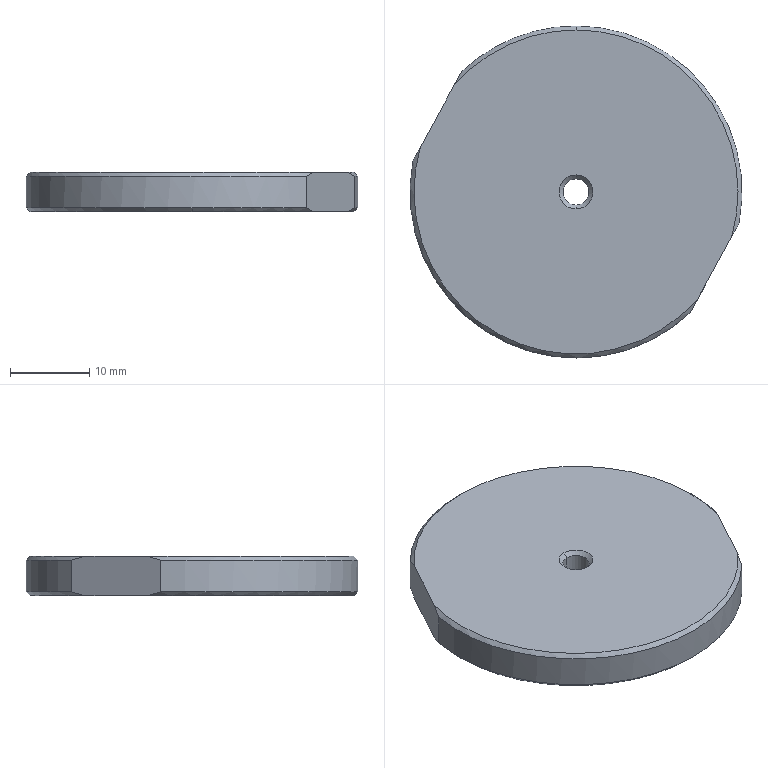Part | SolidWorks | features BaseBody 1 | 1 solid | 19 faces | box 42 x 42 x 5 mm | volume 6769 mm3 | cone 10 | cylinder 5 | plane 4 | commonest cylinder face diameters 42 x3 3.3 x2
STEP:
#1=CARTESIAN_POINT('',(489.266,-55.999,281.248));
#2=VERTEX_POINT('',#1);
#3=CARTESIAN_POINT('',(489.266,-52.699,281.248));
#4=VERTEX_POINT('',#3);
#5=CARTESIAN_POINT('',(489.266,-54.349,281.248));
#6=DIRECTION('',(-0.000000004,0.000000009,-1.));
#7=DIRECTION('',(0.5198,-0.8543,-0.000000009));
#8=AXIS2_PLACEMENT_3D('',#5,#6,#7);
#9=CIRCLE('',#8,1.65);
#10=EDGE_CURVE('',#2,#4,#9,.T.);
#11=ORIENTED_EDGE('',*,*,#10,.F.);
#12=CARTESIAN_POINT('',(489.266,-56.499,280.748));
#13=VERTEX_POINT('',#12);
#14=CARTESIAN_POINT('',(489.266,-56.499,280.748));
#15=DIRECTION('',(-0.000000003,-0.7071,-0.7071));
#16=VECTOR('',#15,1000.);
#17=LINE('',#14,#16);
#18=EDGE_CURVE('',#2,#13,#17,.T.);
#19=ORIENTED_EDGE('',*,*,#18,.T.);
#20=CARTESIAN_POINT('',(489.266,-52.199,280.748));
#21=VERTEX_POINT('',#20);
#22=CARTESIAN_POINT('',(489.266,-54.349,280.748));
#23=DIRECTION('',(0.000000004,-0.000000009,1.));
#24=DIRECTION('',(0.,1.,0.000000009));
#25=AXIS2_PLACEMENT_3D('',#22,#23,#24);
#26=CIRCLE('',#25,2.15);
#27=EDGE_CURVE('',#21,#13,#26,.T.);
#28=ORIENTED_EDGE('',*,*,#27,.F.);
#29=CARTESIAN_POINT('',(489.266,-52.199,280.748));
#30=DIRECTION('',(-0.000000003,0.7071,-0.7071));
#31=VECTOR('',#30,1000.);
#32=LINE('',#29,#31);
#33=EDGE_CURVE('',#4,#21,#32,.T.);
#34=ORIENTED_EDGE('',*,*,#33,.F.);
#35=EDGE_LOOP('',(#11,#19,#28,#34));
#36=FACE_OUTER_BOUND('',#35,.T.);
#37=CARTESIAN_POINT('',(489.266,-54.349,280.748));
#38=DIRECTION('',(-0.000000004,0.000000009,-1.));
#39=DIRECTION('',(0.,1.,0.000000009));
#40=AXIS2_PLACEMENT_3D('',#37,#38,#39);
#41=CONICAL_SURFACE('',#40,2.15,0.7854);
#42=ADVANCED_FACE('',(#36),#41,.F.);
#43=CARTESIAN_POINT('',(489.266,-74.849,280.748));
#44=VERTEX_POINT('',#43);
#45=CARTESIAN_POINT('',(469.56,-48.699,280.748));
#46=VERTEX_POINT('',#45);
#47=CARTESIAN_POINT('',(489.266,-54.349,280.748));
#48=DIRECTION('',(-0.000000004,0.000000009,-1.));
#49=DIRECTION('',(0.,-1.,-0.000000009));
#50=AXIS2_PLACEMENT_3D('',#47,#48,#49);
#51=CIRCLE('',#50,20.5);
#52=EDGE_CURVE('',#44,#46,#51,.T.);
#53=ORIENTED_EDGE('',*,*,#52,.F.);
#54=CARTESIAN_POINT('',(489.266,-75.349,281.248));
#55=VERTEX_POINT('',#54);
#56=CARTESIAN_POINT('',(489.266,-75.349,281.248));
#57=DIRECTION('',(0.000000003,-0.7071,0.7071));
#58=VECTOR('',#57,1000.);
#59=LINE('',#56,#58);
#60=EDGE_CURVE('',#44,#55,#59,.T.);
#61=ORIENTED_EDGE('',*,*,#60,.T.);
#62=CARTESIAN_POINT('',(468.647,-50.368,281.248));
#63=VERTEX_POINT('',#62);
#64=CARTESIAN_POINT('',(489.266,-54.349,281.248));
#65=DIRECTION('',(-0.000000004,0.000000009,-1.));
#66=DIRECTION('',(-0.5198,0.8543,0.000000009));
#67=AXIS2_PLACEMENT_3D('',#64,#65,#66);
#68=CIRCLE('',#67,21.);
#69=EDGE_CURVE('',#55,#63,#68,.T.);
#70=ORIENTED_EDGE('',*,*,#69,.T.);
#71=CARTESIAN_POINT('',(468.647,-50.368,281.248));
#72=CARTESIAN_POINT('',(468.948,-49.818,281.056));
#73=CARTESIAN_POINT('',(469.252,-49.261,280.888));
#74=CARTESIAN_POINT('',(469.56,-48.699,280.748));
#75=B_SPLINE_CURVE_WITH_KNOTS('',3,(#71,#72,#73,#74),.UNSPECIFIED.,.F.,.F.,(4,4),(0.,0.001968),.UNSPECIFIED.);
#76=EDGE_CURVE('',#63,#46,#75,.T.);
#77=ORIENTED_EDGE('',*,*,#76,.T.);
#78=EDGE_LOOP('',(#53,#61,#70,#77));
#79=FACE_OUTER_BOUND('',#78,.T.);
#80=CARTESIAN_POINT('',(489.266,-54.349,281.248));
#81=DIRECTION('',(0.000000004,-0.000000009,1.));
#82=DIRECTION('',(0.,-1.,-0.000000009));
#83=AXIS2_PLACEMENT_3D('',#80,#81,#82);
#84=CONICAL_SURFACE('',#83,21.,0.7854);
#85=ADVANCED_FACE('',(#79),#84,.T.);
#86=ORIENTED_EDGE('',*,*,#10,.T.);
#87=CARTESIAN_POINT('',(489.266,-52.699,285.248));
#88=VERTEX_POINT('',#87);
#89=CARTESIAN_POINT('',(489.266,-52.699,283.748));
#90=DIRECTION('',(0.000000004,-0.000000009,1.));
#91=VECTOR('',#90,1000.);
#92=LINE('',#89,#91);
#93=EDGE_CURVE('',#4,#88,#92,.T.);
#94=ORIENTED_EDGE('',*,*,#93,.T.);
#95=CARTESIAN_POINT('',(489.266,-55.999,285.248));
#96=VERTEX_POINT('',#95);
#97=CARTESIAN_POINT('',(489.266,-54.349,285.248));
#98=DIRECTION('',(-0.000000004,0.000000009,-1.));
#99=DIRECTION('',(0.,-1.,-0.000000009));
#100=AXIS2_PLACEMENT_3D('',#97,#98,#99);
#101=CIRCLE('',#100,1.65);
#102=EDGE_CURVE('',#96,#88,#101,.T.);
#103=ORIENTED_EDGE('',*,*,#102,.F.);
#104=CARTESIAN_POINT('',(489.266,-55.999,283.748));
#105=DIRECTION('',(0.000000004,-0.000000009,1.));
#106=VECTOR('',#105,1000.);
#107=LINE('',#104,#106);
#108=EDGE_CURVE('',#2,#96,#107,.T.);
#109=ORIENTED_EDGE('',*,*,#108,.F.);
#110=EDGE_LOOP('',(#86,#94,#103,#109));
#111=FACE_OUTER_BOUND('',#110,.T.);
#112=CARTESIAN_POINT('',(489.266,-54.349,283.748));
#113=DIRECTION('',(0.000000004,-0.000000009,1.));
#114=DIRECTION('',(0.,-1.,-0.000000009));
#115=AXIS2_PLACEMENT_3D('',#112,#113,#114);
#116=CYLINDRICAL_SURFACE('',#115,1.65);
#117=ADVANCED_FACE('',(#111),#116,.F.);
#118=CARTESIAN_POINT('',(474.792,-39.133,285.248));
#119=VERTEX_POINT('',#118);
#120=CARTESIAN_POINT('',(489.266,-33.349,285.248));
#121=VERTEX_POINT('',#120);
#122=CARTESIAN_POINT('',(489.266,-54.349,285.248));
#123=DIRECTION('',(-0.000000004,0.000000009,-1.));
#124=DIRECTION('',(0.,1.,0.000000009));
#125=AXIS2_PLACEMENT_3D('',#122,#123,#124);
#126=CIRCLE('',#125,21.);
#127=EDGE_CURVE('',#119,#121,#126,.T.);
#128=ORIENTED_EDGE('',*,*,#127,.T.);
#129=CARTESIAN_POINT('',(489.266,-33.349,281.248));
#130=VERTEX_POINT('',#129);
#131=CARTESIAN_POINT('',(489.266,-33.349,285.748));
#132=DIRECTION('',(-0.000000004,0.000000009,-1.));
#133=VECTOR('',#132,1000.);
#134=LINE('',#131,#133);
#135=EDGE_CURVE('',#121,#130,#134,.T.);
#136=ORIENTED_EDGE('',*,*,#135,.T.);
#137=CARTESIAN_POINT('',(474.792,-39.133,281.248));
#138=VERTEX_POINT('',#137);
#139=CARTESIAN_POINT('',(489.266,-54.349,281.248));
#140=DIRECTION('',(-0.000000004,0.000000009,-1.));
#141=DIRECTION('',(-0.5198,0.8543,0.000000009));
#142=AXIS2_PLACEMENT_3D('',#139,#140,#141);
#143=CIRCLE('',#142,21.);
#144=EDGE_CURVE('',#138,#130,#143,.T.);
#145=ORIENTED_EDGE('',*,*,#144,.F.);
#146=CARTESIAN_POINT('',(474.792,-39.133,285.748));
#147=DIRECTION('',(0.000000007,-0.000000004,1.));
#148=VECTOR('',#147,1000.);
#149=LINE('',#146,#148);
#150=EDGE_CURVE('',#138,#119,#149,.T.);
#151=ORIENTED_EDGE('',*,*,#150,.T.);
#152=EDGE_LOOP('',(#128,#136,#145,#151));
#153=FACE_OUTER_BOUND('',#152,.T.);
#154=CARTESIAN_POINT('',(489.266,-54.349,285.748));
#155=DIRECTION('',(-0.000000004,0.000000009,-1.));
#156=DIRECTION('',(0.,1.,0.000000009));
#157=AXIS2_PLACEMENT_3D('',#154,#155,#156);
#158=CYLINDRICAL_SURFACE('',#157,21.);
#159=ADVANCED_FACE('',(#153),#158,.T.);
#160=CARTESIAN_POINT('',(473.879,-40.803,285.748));
#161=VERTEX_POINT('',#160);
#162=CARTESIAN_POINT('',(489.266,-33.849,285.748));
#163=VERTEX_POINT('',#162);
#164=CARTESIAN_POINT('',(489.266,-54.349,285.748));
#165=DIRECTION('',(-0.000000004,0.000000009,-1.));
#166=DIRECTION('',(0.,1.,0.000000009));
#167=AXIS2_PLACEMENT_3D('',#164,#165,#166);
#168=CIRCLE('',#167,20.5);
#169=EDGE_CURVE('',#161,#163,#168,.T.);
#170=ORIENTED_EDGE('',*,*,#169,.T.);
#171=CARTESIAN_POINT('',(489.266,-33.349,285.248));
#172=DIRECTION('',(-0.000000003,0.7071,-0.7071));
#173=VECTOR('',#172,1000.);
#174=LINE('',#171,#173);
#175=EDGE_CURVE('',#163,#121,#174,.T.);
#176=ORIENTED_EDGE('',*,*,#175,.T.);
#177=ORIENTED_EDGE('',*,*,#127,.F.);
#178=CARTESIAN_POINT('',(474.792,-39.133,285.248));
#179=CARTESIAN_POINT('',(474.491,-39.684,285.439));
#180=CARTESIAN_POINT('',(474.187,-40.24,285.607));
#181=CARTESIAN_POINT('',(473.879,-40.803,285.748));
#182=B_SPLINE_CURVE_WITH_KNOTS('',3,(#178,#179,#180,#181),.UNSPECIFIED.,.F.,.F.,(4,4),(0.,0.001968),.UNSPECIFIED.);
#183=EDGE_CURVE('',#119,#161,#182,.T.);
#184=ORIENTED_EDGE('',*,*,#183,.T.);
#185=EDGE_LOOP('',(#170,#176,#177,#184));
#186=FACE_OUTER_BOUND('',#185,.T.);
#187=CARTESIAN_POINT('',(489.266,-54.349,285.248));
#188=DIRECTION('',(-0.000000004,0.000000009,-1.));
#189=DIRECTION('',(0.,1.,0.000000009));
#190=AXIS2_PLACEMENT_3D('',#187,#188,#189);
#191=CONICAL_SURFACE('',#190,21.,0.7854);
#192=ADVANCED_FACE('',(#186),#191,.T.);
#193=ORIENTED_EDGE('',*,*,#102,.T.);
#194=CARTESIAN_POINT('',(489.266,-52.199,285.748));
#195=VERTEX_POINT('',#194);
#196=CARTESIAN_POINT('',(489.266,-52.199,285.748));
#197=DIRECTION('',(0.000000003,0.7071,0.7071));
#198=VECTOR('',#197,1000.);
#199=LINE('',#196,#198);
#200=EDGE_CURVE('',#88,#195,#199,.T.);
#201=ORIENTED_EDGE('',*,*,#200,.T.);
#202=CARTESIAN_POINT('',(489.266,-56.499,285.748));
#203=VERTEX_POINT('',#202);
#204=CARTESIAN_POINT('',(489.266,-54.349,285.748));
#205=DIRECTION('',(0.000000004,-0.000000009,1.));
#206=DIRECTION('',(0.,-1.,-0.000000009));
#207=AXIS2_PLACEMENT_3D('',#204,#205,#206);
#208=CIRCLE('',#207,2.15);
#209=EDGE_CURVE('',#195,#203,#208,.T.);
#210=ORIENTED_EDGE('',*,*,#209,.T.);
#211=CARTESIAN_POINT('',(489.266,-56.499,285.748));
#212=DIRECTION('',(0.000000003,-0.7071,0.7071));
#213=VECTOR('',#212,1000.);
#214=LINE('',#211,#213);
#215=EDGE_CURVE('',#96,#203,#214,.T.);
#216=ORIENTED_EDGE('',*,*,#215,.F.);
#217=EDGE_LOOP('',(#193,#201,#210,#216));
#218=FACE_OUTER_BOUND('',#217,.T.);
#219=CARTESIAN_POINT('',(489.266,-54.349,285.748));
#220=DIRECTION('',(0.000000004,-0.000000009,1.));
#221=DIRECTION('',(0.,-1.,-0.000000009));
#222=AXIS2_PLACEMENT_3D('',#219,#220,#221);
#223=CONICAL_SURFACE('',#222,2.15,0.7854);
#224=ADVANCED_FACE('',(#218),#223,.F.);
#225=ORIENTED_EDGE('',*,*,#27,.T.);
#226=CARTESIAN_POINT('',(489.266,-54.349,280.748));
#227=DIRECTION('',(0.000000004,-0.000000009,1.));
#228=DIRECTION('',(0.,1.,0.000000009));
#229=AXIS2_PLACEMENT_3D('',#226,#227,#228);
#230=CIRCLE('',#229,2.15);
#231=EDGE_CURVE('',#13,#21,#230,.T.);
#232=ORIENTED_EDGE('',*,*,#231,.T.);
#233=EDGE_LOOP('',(#225,#232));
#234=FACE_BOUND('',#233,.T.);
#235=CARTESIAN_POINT('',(473.879,-40.803,280.748));
#236=VERTEX_POINT('',#235);
#237=CARTESIAN_POINT('',(508.972,-59.999,280.748));
#238=VERTEX_POINT('',#237);
#239=CARTESIAN_POINT('',(489.266,-54.349,280.748));
#240=DIRECTION('',(-0.000000004,0.000000009,-1.));
#241=DIRECTION('',(0.,-1.,-0.000000009));
#242=AXIS2_PLACEMENT_3D('',#239,#240,#241);
#243=CIRCLE('',#242,20.5);
#244=EDGE_CURVE('',#236,#238,#243,.T.);
#245=ORIENTED_EDGE('',*,*,#244,.T.);
#246=CARTESIAN_POINT('',(504.653,-67.895,280.748));
#247=VERTEX_POINT('',#246);
#248=CARTESIAN_POINT('',(508.972,-59.999,280.748));
#249=DIRECTION('',(-0.4799,-0.8773,-0.000000006));
#250=VECTOR('',#249,1000.);
#251=LINE('',#248,#250);
#252=EDGE_CURVE('',#238,#247,#251,.T.);
#253=ORIENTED_EDGE('',*,*,#252,.T.);
#254=CARTESIAN_POINT('',(489.266,-54.349,280.748));
#255=DIRECTION('',(-0.000000004,0.000000009,-1.));
#256=DIRECTION('',(0.,-1.,-0.000000009));
#257=AXIS2_PLACEMENT_3D('',#254,#255,#256);
#258=CIRCLE('',#257,20.5);
#259=EDGE_CURVE('',#247,#44,#258,.T.);
#260=ORIENTED_EDGE('',*,*,#259,.T.);
#261=ORIENTED_EDGE('',*,*,#52,.T.);
#262=CARTESIAN_POINT('',(469.56,-48.699,280.748));
#263=DIRECTION('',(0.4799,0.8773,0.000000006));
#264=VECTOR('',#263,1000.);
#265=LINE('',#262,#264);
#266=EDGE_CURVE('',#46,#236,#265,.T.);
#267=ORIENTED_EDGE('',*,*,#266,.T.);
#268=EDGE_LOOP('',(#245,#253,#260,#261,#267));
#269=FACE_OUTER_BOUND('',#268,.T.);
#270=CARTESIAN_POINT('',(489.266,-54.349,280.748));
#271=DIRECTION('',(-0.000000004,0.000000009,-1.));
#272=DIRECTION('',(0.,1.,0.000000009));
#273=AXIS2_PLACEMENT_3D('',#270,#271,#272);
#274=PLANE('',#273);
#275=ADVANCED_FACE('',(#234,#269),#274,.T.);
#276=ORIENTED_EDGE('',*,*,#18,.F.);
#277=CARTESIAN_POINT('',(489.266,-54.349,281.248));
#278=DIRECTION('',(-0.000000004,0.000000009,-1.));
#279=DIRECTION('',(0.5198,-0.8543,-0.000000009));
#280=AXIS2_PLACEMENT_3D('',#277,#278,#279);
#281=CIRCLE('',#280,1.65);
#282=EDGE_CURVE('',#4,#2,#281,.T.);
#283=ORIENTED_EDGE('',*,*,#282,.F.);
#284=ORIENTED_EDGE('',*,*,#33,.T.);
#285=ORIENTED_EDGE('',*,*,#231,.F.);
#286=EDGE_LOOP('',(#276,#283,#284,#285));
#287=FACE_OUTER_BOUND('',#286,.T.);
#288=CARTESIAN_POINT('',(489.266,-54.349,280.748));
#289=DIRECTION('',(-0.000000004,0.000000009,-1.));
#290=DIRECTION('',(0.,1.,0.000000009));
#291=AXIS2_PLACEMENT_3D('',#288,#289,#290);
#292=CONICAL_SURFACE('',#291,2.15,0.7854);
#293=ADVANCED_FACE('',(#287),#292,.F.);
#294=CARTESIAN_POINT('',(509.885,-58.33,281.248));
#295=VERTEX_POINT('',#294);
#296=CARTESIAN_POINT('',(509.885,-58.33,281.248));
#297=CARTESIAN_POINT('',(509.584,-58.881,281.056));
#298=CARTESIAN_POINT('',(509.28,-59.437,280.888));
#299=CARTESIAN_POINT('',(508.972,-59.999,280.748));
#300=B_SPLINE_CURVE_WITH_KNOTS('',3,(#296,#297,#298,#299),.UNSPECIFIED.,.F.,.F.,(4,4),(0.,0.001968),.UNSPECIFIED.);
#301=EDGE_CURVE('',#295,#238,#300,.T.);
#302=ORIENTED_EDGE('',*,*,#301,.T.);
#303=ORIENTED_EDGE('',*,*,#244,.F.);
#304=CARTESIAN_POINT('',(473.879,-40.803,280.748));
#305=CARTESIAN_POINT('',(474.187,-40.24,280.888));
#306=CARTESIAN_POINT('',(474.491,-39.684,281.056));
#307=CARTESIAN_POINT('',(474.792,-39.133,281.248));
#308=B_SPLINE_CURVE_WITH_KNOTS('',3,(#304,#305,#306,#307),.UNSPECIFIED.,.F.,.F.,(4,4),(0.,0.001968),.UNSPECIFIED.);
#309=EDGE_CURVE('',#236,#138,#308,.T.);
#310=ORIENTED_EDGE('',*,*,#309,.T.);
#311=ORIENTED_EDGE('',*,*,#144,.T.);
#312=CARTESIAN_POINT('',(489.266,-54.349,281.248));
#313=DIRECTION('',(-0.000000004,0.000000009,-1.));
#314=DIRECTION('',(-0.5198,0.8543,0.000000009));
#315=AXIS2_PLACEMENT_3D('',#312,#313,#314);
#316=CIRCLE('',#315,21.);
#317=EDGE_CURVE('',#130,#295,#316,.T.);
#318=ORIENTED_EDGE('',*,*,#317,.T.);
#319=EDGE_LOOP('',(#302,#303,#310,#311,#318));
#320=FACE_OUTER_BOUND('',#319,.T.);
#321=CARTESIAN_POINT('',(489.266,-54.349,281.248));
#322=DIRECTION('',(0.000000004,-0.000000009,1.));
#323=DIRECTION('',(0.,-1.,-0.000000009));
#324=AXIS2_PLACEMENT_3D('',#321,#322,#323);
#325=CONICAL_SURFACE('',#324,21.,0.7854);
#326=ADVANCED_FACE('',(#320),#325,.T.);
#327=ORIENTED_EDGE('',*,*,#150,.F.);
#328=ORIENTED_EDGE('',*,*,#309,.F.);
#329=ORIENTED_EDGE('',*,*,#266,.F.);
#330=ORIENTED_EDGE('',*,*,#76,.F.);
#331=CARTESIAN_POINT('',(468.647,-50.368,285.248));
#332=VERTEX_POINT('',#331);
#333=CARTESIAN_POINT('',(468.647,-50.368,285.748));
#334=DIRECTION('',(-0.000000007,0.000000004,-1.));
#335=VECTOR('',#334,1000.);
#336=LINE('',#333,#335);
#337=EDGE_CURVE('',#332,#63,#336,.T.);
#338=ORIENTED_EDGE('',*,*,#337,.F.);
#339=CARTESIAN_POINT('',(469.56,-48.699,285.748));
#340=VERTEX_POINT('',#339);
#341=CARTESIAN_POINT('',(469.56,-48.699,285.748));
#342=CARTESIAN_POINT('',(469.252,-49.261,285.607));
#343=CARTESIAN_POINT('',(468.948,-49.818,285.439));
#344=CARTESIAN_POINT('',(468.647,-50.368,285.248));
#345=B_SPLINE_CURVE_WITH_KNOTS('',3,(#341,#342,#343,#344),.UNSPECIFIED.,.F.,.F.,(4,4),(0.,0.001968),.UNSPECIFIED.);
#346=EDGE_CURVE('',#340,#332,#345,.T.);
#347=ORIENTED_EDGE('',*,*,#346,.F.);
#348=CARTESIAN_POINT('',(468.647,-50.368,285.748));
#349=DIRECTION('',(-0.4799,-0.8773,0.));
#350=VECTOR('',#349,1000.);
#351=LINE('',#348,#350);
#352=EDGE_CURVE('',#161,#340,#351,.T.);
#353=ORIENTED_EDGE('',*,*,#352,.F.);
#354=ORIENTED_EDGE('',*,*,#183,.F.);
#355=EDGE_LOOP('',(#327,#328,#329,#330,#338,#347,#353,#354));
#356=FACE_OUTER_BOUND('',#355,.T.);
#357=CARTESIAN_POINT('',(468.647,-50.368,285.748));
#358=DIRECTION('',(0.8773,-0.4799,-0.000000008));
#359=DIRECTION('',(0.4799,0.8773,0.));
#360=AXIS2_PLACEMENT_3D('',#357,#358,#359);
#361=PLANE('',#360);
#362=ADVANCED_FACE('',(#356),#361,.F.);
#363=ORIENTED_EDGE('',*,*,#60,.F.);
#364=ORIENTED_EDGE('',*,*,#259,.F.);
#365=CARTESIAN_POINT('',(503.739,-69.565,281.248));
#366=VERTEX_POINT('',#365);
#367=CARTESIAN_POINT('',(504.653,-67.895,280.748));
#368=CARTESIAN_POINT('',(504.345,-68.458,280.888));
#369=CARTESIAN_POINT('',(504.041,-69.014,281.056));
#370=CARTESIAN_POINT('',(503.739,-69.565,281.248));
#371=B_SPLINE_CURVE_WITH_KNOTS('',3,(#367,#368,#369,#370),.UNSPECIFIED.,.F.,.F.,(4,4),(0.,0.001968),.UNSPECIFIED.);
#372=EDGE_CURVE('',#247,#366,#371,.T.);
#373=ORIENTED_EDGE('',*,*,#372,.T.);
#374=CARTESIAN_POINT('',(489.266,-54.349,281.248));
#375=DIRECTION('',(-0.000000004,0.000000009,-1.));
#376=DIRECTION('',(-0.5198,0.8543,0.000000009));
#377=AXIS2_PLACEMENT_3D('',#374,#375,#376);
#378=CIRCLE('',#377,21.);
#379=EDGE_CURVE('',#366,#55,#378,.T.);
#380=ORIENTED_EDGE('',*,*,#379,.T.);
#381=EDGE_LOOP('',(#363,#364,#373,#380));
#382=FACE_OUTER_BOUND('',#381,.T.);
#383=CARTESIAN_POINT('',(489.266,-54.349,281.248));
#384=DIRECTION('',(0.000000004,-0.000000009,1.));
#385=DIRECTION('',(0.,-1.,-0.000000009));
#386=AXIS2_PLACEMENT_3D('',#383,#384,#385);
#387=CONICAL_SURFACE('',#386,21.,0.7854);
#388=ADVANCED_FACE('',(#382),#387,.T.);
#389=CARTESIAN_POINT('',(503.739,-69.565,285.248));
#390=VERTEX_POINT('',#389);
#391=CARTESIAN_POINT('',(503.739,-69.565,285.748));
#392=DIRECTION('',(0.000000007,-0.000000004,1.));
#393=VECTOR('',#392,1000.);
#394=LINE('',#391,#393);
#395=EDGE_CURVE('',#366,#390,#394,.T.);
#396=ORIENTED_EDGE('',*,*,#395,.F.);
#397=ORIENTED_EDGE('',*,*,#372,.F.);
#398=ORIENTED_EDGE('',*,*,#252,.F.);
#399=ORIENTED_EDGE('',*,*,#301,.F.);
#400=CARTESIAN_POINT('',(509.885,-58.33,285.248));
#401=VERTEX_POINT('',#400);
#402=CARTESIAN_POINT('',(509.885,-58.33,285.748));
#403=DIRECTION('',(-0.000000007,0.000000004,-1.));
#404=VECTOR('',#403,1000.);
#405=LINE('',#402,#404);
#406=EDGE_CURVE('',#401,#295,#405,.T.);
#407=ORIENTED_EDGE('',*,*,#406,.F.);
#408=CARTESIAN_POINT('',(508.972,-59.999,285.748));
#409=VERTEX_POINT('',#408);
#410=CARTESIAN_POINT('',(508.972,-59.999,285.748));
#411=CARTESIAN_POINT('',(509.28,-59.437,285.607));
#412=CARTESIAN_POINT('',(509.584,-58.881,285.439));
#413=CARTESIAN_POINT('',(509.885,-58.33,285.248));
#414=B_SPLINE_CURVE_WITH_KNOTS('',3,(#410,#411,#412,#413),.UNSPECIFIED.,.F.,.F.,(4,4),(0.,0.001968),.UNSPECIFIED.);
#415=EDGE_CURVE('',#409,#401,#414,.T.);
#416=ORIENTED_EDGE('',*,*,#415,.F.);
#417=CARTESIAN_POINT('',(504.653,-67.895,285.748));
#418=VERTEX_POINT('',#417);
#419=CARTESIAN_POINT('',(509.885,-58.33,285.748));
#420=DIRECTION('',(0.4799,0.8773,0.));
#421=VECTOR('',#420,1000.);
#422=LINE('',#419,#421);
#423=EDGE_CURVE('',#418,#409,#422,.T.);
#424=ORIENTED_EDGE('',*,*,#423,.F.);
#425=CARTESIAN_POINT('',(503.739,-69.565,285.248));
#426=CARTESIAN_POINT('',(504.041,-69.014,285.439));
#427=CARTESIAN_POINT('',(504.345,-68.458,285.607));
#428=CARTESIAN_POINT('',(504.653,-67.895,285.748));
#429=B_SPLINE_CURVE_WITH_KNOTS('',3,(#425,#426,#427,#428),.UNSPECIFIED.,.F.,.F.,(4,4),(0.,0.001968),.UNSPECIFIED.);
#430=EDGE_CURVE('',#390,#418,#429,.T.);
#431=ORIENTED_EDGE('',*,*,#430,.F.);
#432=EDGE_LOOP('',(#396,#397,#398,#399,#407,#416,#424,#431));
#433=FACE_OUTER_BOUND('',#432,.T.);
#434=CARTESIAN_POINT('',(509.885,-58.33,285.748));
#435=DIRECTION('',(-0.8773,0.4799,0.000000008));
#436=DIRECTION('',(-0.4799,-0.8773,0.));
#437=AXIS2_PLACEMENT_3D('',#434,#435,#436);
#438=PLANE('',#437);
#439=ADVANCED_FACE('',(#433),#438,.F.);
#440=ORIENTED_EDGE('',*,*,#93,.F.);
#441=ORIENTED_EDGE('',*,*,#282,.T.);
#442=ORIENTED_EDGE('',*,*,#108,.T.);
#443=CARTESIAN_POINT('',(489.266,-54.349,285.248));
#444=DIRECTION('',(-0.000000004,0.000000009,-1.));
#445=DIRECTION('',(0.,-1.,-0.000000009));
#446=AXIS2_PLACEMENT_3D('',#443,#444,#445);
#447=CIRCLE('',#446,1.65);
#448=EDGE_CURVE('',#88,#96,#447,.T.);
#449=ORIENTED_EDGE('',*,*,#448,.F.);
#450=EDGE_LOOP('',(#440,#441,#442,#449));
#451=FACE_OUTER_BOUND('',#450,.T.);
#452=CARTESIAN_POINT('',(489.266,-54.349,283.748));
#453=DIRECTION('',(0.000000004,-0.000000009,1.));
#454=DIRECTION('',(0.,-1.,-0.000000009));
#455=AXIS2_PLACEMENT_3D('',#452,#453,#454);
#456=CYLINDRICAL_SURFACE('',#455,1.65);
#457=ADVANCED_FACE('',(#451),#456,.F.);
#458=ORIENTED_EDGE('',*,*,#135,.F.);
#459=CARTESIAN_POINT('',(489.266,-54.349,285.248));
#460=DIRECTION('',(-0.000000004,0.000000009,-1.));
#461=DIRECTION('',(0.,1.,0.000000009));
#462=AXIS2_PLACEMENT_3D('',#459,#460,#461);
#463=CIRCLE('',#462,21.);
#464=EDGE_CURVE('',#121,#401,#463,.T.);
#465=ORIENTED_EDGE('',*,*,#464,.T.);
#466=ORIENTED_EDGE('',*,*,#406,.T.);
#467=ORIENTED_EDGE('',*,*,#317,.F.);
#468=EDGE_LOOP('',(#458,#465,#466,#467));
#469=FACE_OUTER_BOUND('',#468,.T.);
#470=CARTESIAN_POINT('',(489.266,-54.349,285.748));
#471=DIRECTION('',(-0.000000004,0.000000009,-1.));
#472=DIRECTION('',(0.,1.,0.000000009));
#473=AXIS2_PLACEMENT_3D('',#470,#471,#472);
#474=CYLINDRICAL_SURFACE('',#473,21.);
#475=ADVANCED_FACE('',(#469),#474,.T.);
#476=ORIENTED_EDGE('',*,*,#175,.F.);
#477=CARTESIAN_POINT('',(489.266,-54.349,285.748));
#478=DIRECTION('',(-0.000000004,0.000000009,-1.));
#479=DIRECTION('',(0.,1.,0.000000009));
#480=AXIS2_PLACEMENT_3D('',#477,#478,#479);
#481=CIRCLE('',#480,20.5);
#482=EDGE_CURVE('',#163,#409,#481,.T.);
#483=ORIENTED_EDGE('',*,*,#482,.T.);
#484=ORIENTED_EDGE('',*,*,#415,.T.);
#485=ORIENTED_EDGE('',*,*,#464,.F.);
#486=EDGE_LOOP('',(#476,#483,#484,#485));
#487=FACE_OUTER_BOUND('',#486,.T.);
#488=CARTESIAN_POINT('',(489.266,-54.349,285.248));
#489=DIRECTION('',(-0.000000004,0.000000009,-1.));
#490=DIRECTION('',(0.,1.,0.000000009));
#491=AXIS2_PLACEMENT_3D('',#488,#489,#490);
#492=CONICAL_SURFACE('',#491,21.,0.7854);
#493=ADVANCED_FACE('',(#487),#492,.T.);
#494=ORIENTED_EDGE('',*,*,#337,.T.);
#495=ORIENTED_EDGE('',*,*,#69,.F.);
#496=ORIENTED_EDGE('',*,*,#379,.F.);
#497=ORIENTED_EDGE('',*,*,#395,.T.);
#498=CARTESIAN_POINT('',(489.266,-54.349,285.248));
#499=DIRECTION('',(-0.000000004,0.000000009,-1.));
#500=DIRECTION('',(0.,1.,0.000000009));
#501=AXIS2_PLACEMENT_3D('',#498,#499,#500);
#502=CIRCLE('',#501,21.);
#503=EDGE_CURVE('',#390,#332,#502,.T.);
#504=ORIENTED_EDGE('',*,*,#503,.T.);
#505=EDGE_LOOP('',(#494,#495,#496,#497,#504));
#506=FACE_OUTER_BOUND('',#505,.T.);
#507=CARTESIAN_POINT('',(489.266,-54.349,285.748));
#508=DIRECTION('',(-0.000000004,0.000000009,-1.));
#509=DIRECTION('',(0.,1.,0.000000009));
#510=AXIS2_PLACEMENT_3D('',#507,#508,#509);
#511=CYLINDRICAL_SURFACE('',#510,21.);
#512=ADVANCED_FACE('',(#506),#511,.T.);
#513=ORIENTED_EDGE('',*,*,#346,.T.);
#514=ORIENTED_EDGE('',*,*,#503,.F.);
#515=ORIENTED_EDGE('',*,*,#430,.T.);
#516=CARTESIAN_POINT('',(489.266,-54.349,285.748));
#517=DIRECTION('',(-0.000000004,0.000000009,-1.));
#518=DIRECTION('',(0.,1.,0.000000009));
#519=AXIS2_PLACEMENT_3D('',#516,#517,#518);
#520=CIRCLE('',#519,20.5);
#521=EDGE_CURVE('',#418,#340,#520,.T.);
#522=ORIENTED_EDGE('',*,*,#521,.T.);
#523=EDGE_LOOP('',(#513,#514,#515,#522));
#524=FACE_OUTER_BOUND('',#523,.T.);
#525=CARTESIAN_POINT('',(489.266,-54.349,285.248));
#526=DIRECTION('',(-0.000000004,0.000000009,-1.));
#527=DIRECTION('',(0.,1.,0.000000009));
#528=AXIS2_PLACEMENT_3D('',#525,#526,#527);
#529=CONICAL_SURFACE('',#528,21.,0.7854);
#530=ADVANCED_FACE('',(#524),#529,.T.);
#531=CARTESIAN_POINT('',(489.266,-54.349,285.748));
#532=DIRECTION('',(0.000000004,-0.000000009,1.));
#533=DIRECTION('',(0.,-1.,-0.000000009));
#534=AXIS2_PLACEMENT_3D('',#531,#532,#533);
#535=CIRCLE('',#534,2.15);
#536=EDGE_CURVE('',#203,#195,#535,.T.);
#537=ORIENTED_EDGE('',*,*,#536,.F.);
#538=ORIENTED_EDGE('',*,*,#209,.F.);
#539=EDGE_LOOP('',(#537,#538));
#540=FACE_BOUND('',#539,.T.);
#541=ORIENTED_EDGE('',*,*,#423,.T.);
#542=ORIENTED_EDGE('',*,*,#482,.F.);
#543=ORIENTED_EDGE('',*,*,#169,.F.);
#544=ORIENTED_EDGE('',*,*,#352,.T.);
#545=ORIENTED_EDGE('',*,*,#521,.F.);
#546=EDGE_LOOP('',(#541,#542,#543,#544,#545));
#547=FACE_OUTER_BOUND('',#546,.T.);
#548=CARTESIAN_POINT('',(489.266,-54.349,285.748));
#549=DIRECTION('',(-0.000000004,0.000000009,-1.));
#550=DIRECTION('',(0.,1.,0.000000009));
#551=AXIS2_PLACEMENT_3D('',#548,#549,#550);
#552=PLANE('',#551);
#553=ADVANCED_FACE('',(#540,#547),#552,.F.);
#554=ORIENTED_EDGE('',*,*,#200,.F.);
#555=ORIENTED_EDGE('',*,*,#448,.T.);
#556=ORIENTED_EDGE('',*,*,#215,.T.);
#557=ORIENTED_EDGE('',*,*,#536,.T.);
#558=EDGE_LOOP('',(#554,#555,#556,#557));
#559=FACE_OUTER_BOUND('',#558,.T.);
#560=CARTESIAN_POINT('',(489.266,-54.349,285.748));
#561=DIRECTION('',(0.000000004,-0.000000009,1.));
#562=DIRECTION('',(0.,-1.,-0.000000009));
#563=AXIS2_PLACEMENT_3D('',#560,#561,#562);
#564=CONICAL_SURFACE('',#563,2.15,0.7854);
#565=ADVANCED_FACE('',(#559),#564,.F.);
#566=CLOSED_SHELL('',(#42,#85,#117,#159,#192,#224,#275,#293,#326,#362,#388,#439,#457,#475,#493,#512,#530,#553,#565));
#567=MANIFOLD_SOLID_BREP('',#566);
#568=CARTESIAN_POINT('',(0.,0.,0.));
#569=DIRECTION('',(0.,0.,1.));
#570=DIRECTION('',(1.,0.,0.));
#571=AXIS2_PLACEMENT_3D('',#568,#569,#570);
#572=(LENGTH_UNIT()NAMED_UNIT(*)SI_UNIT(.MILLI.,.METRE.));
#573=UNCERTAINTY_MEASURE_WITH_UNIT(LENGTH_MEASURE(0.00001),#572,'','');
#574=(NAMED_UNIT(*)PLANE_ANGLE_UNIT()SI_UNIT($,.RADIAN.));
#575=(NAMED_UNIT(*)SI_UNIT($,.STERADIAN.)SOLID_ANGLE_UNIT());
#576=(GEOMETRIC_REPRESENTATION_CONTEXT(3)GLOBAL_UNCERTAINTY_ASSIGNED_CONTEXT((#573))GLOBAL_UNIT_ASSIGNED_CONTEXT((#572,#574,#575))REPRESENTATION_CONTEXT('',''));
#577=ADVANCED_BREP_SHAPE_REPRESENTATION('',(#567,#571),#576);